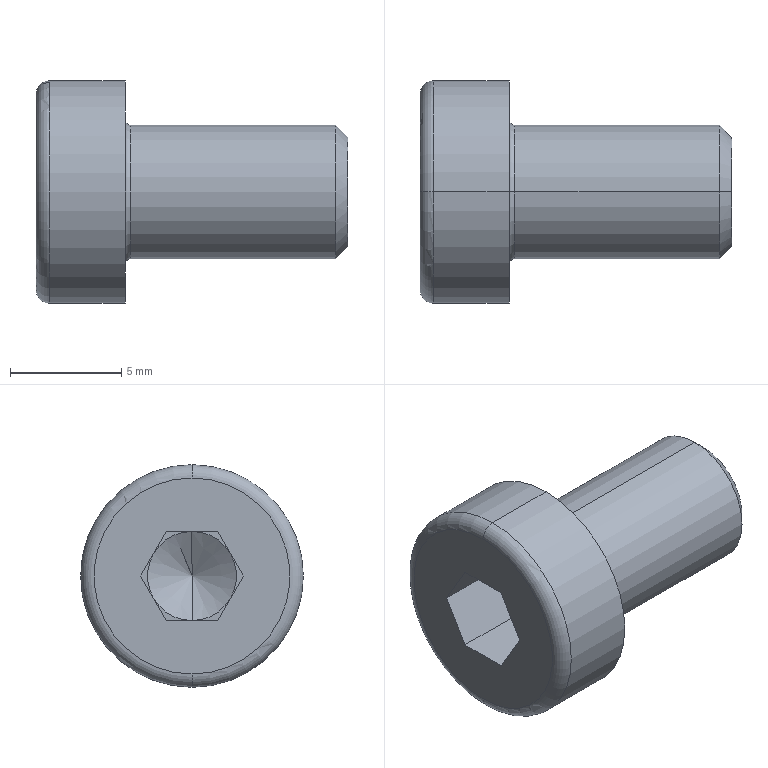Part | STEP file | socket head thin cap screw_din_DIN 7984 - M6 x 10 --- 7N | 1 solid | 27 faces | box 14 x 10 x 10 mm | volume 545.673 mm3 | plane 15 | cone 4 | torus 4 | cylinder 4 | commonest cylinder face diameters 6 x2 10 x2